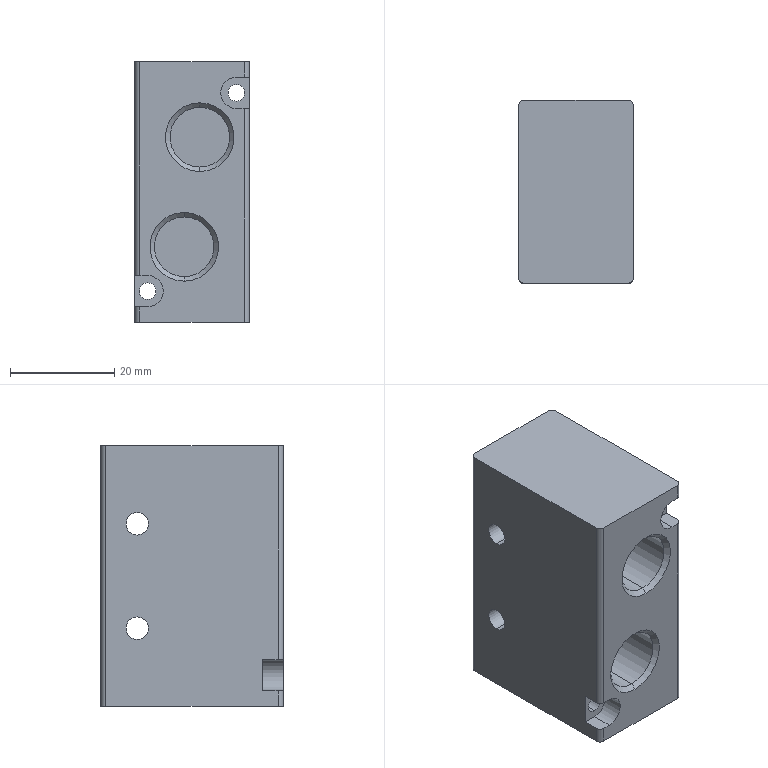Part | STEP file | 1 solid | 53 faces | box 22 x 35 x 50 mm | volume 32799 mm3 | cylinder 26 | plane 17 | cone 10 | commonest cylinder face diameters 2 x6 11.445 x6 3.2 x4 4.3 x4 8.566 x4 6 x2